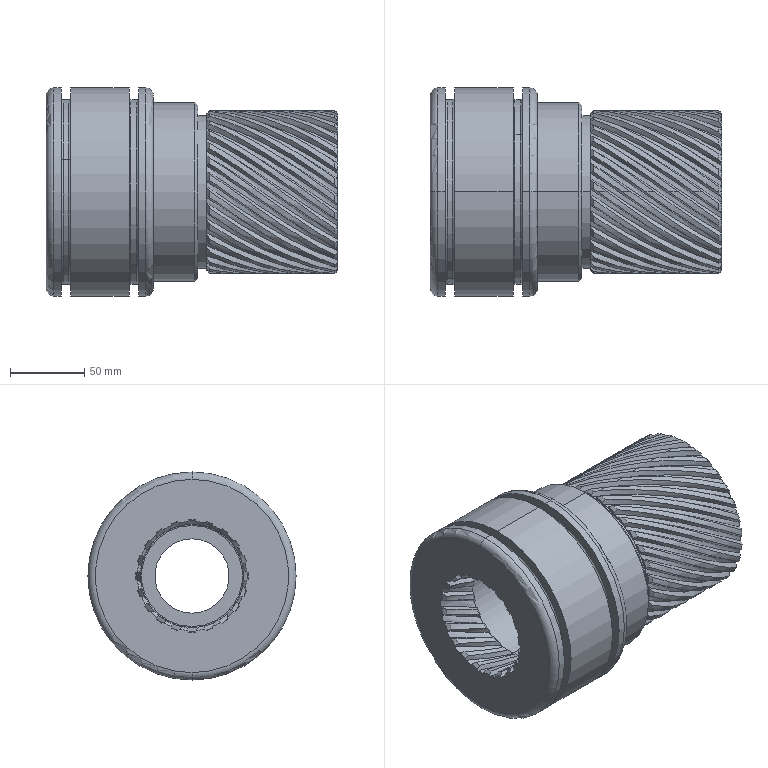Part | SolidWorks | features ICE 6, Cavity 2, Chamfer 2, CirPattern 2, Fillet 2, Helix 2, SweepCut 2, Extrusion 1 | 1 solid | 366 faces | box 196 x 140 x 140 mm | volume 1596152 mm3 | spline 150 | cone 104 | cylinder 83 | plane 15 | torus 14 | commonest cylinder face diameters 110 x36 69.5 x21 50 x6 140 x6 60 x4 124.5 x4